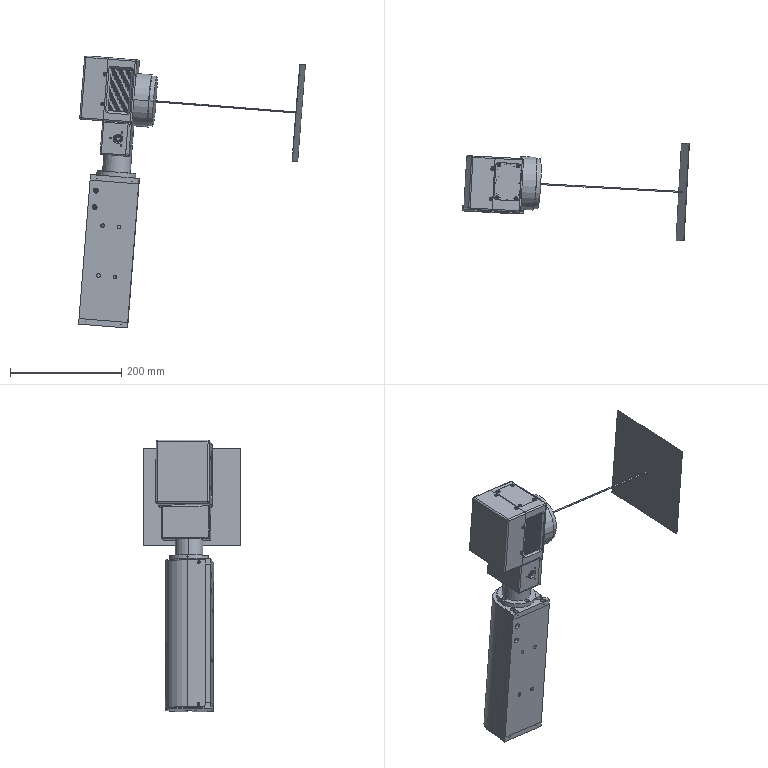Part | SolidWorks | 23 solids | 1130 faces | box 408.184 x 175.143 x 489.463 mm | volume 1754817 mm3 | cylinder 552 | plane 409 | cone 148 | sphere 12 | spline 9 | commonest cylinder face diameters 2.5 x54 3.3 x44 3.5 x42 8 x35 4.2 x34 5 x34